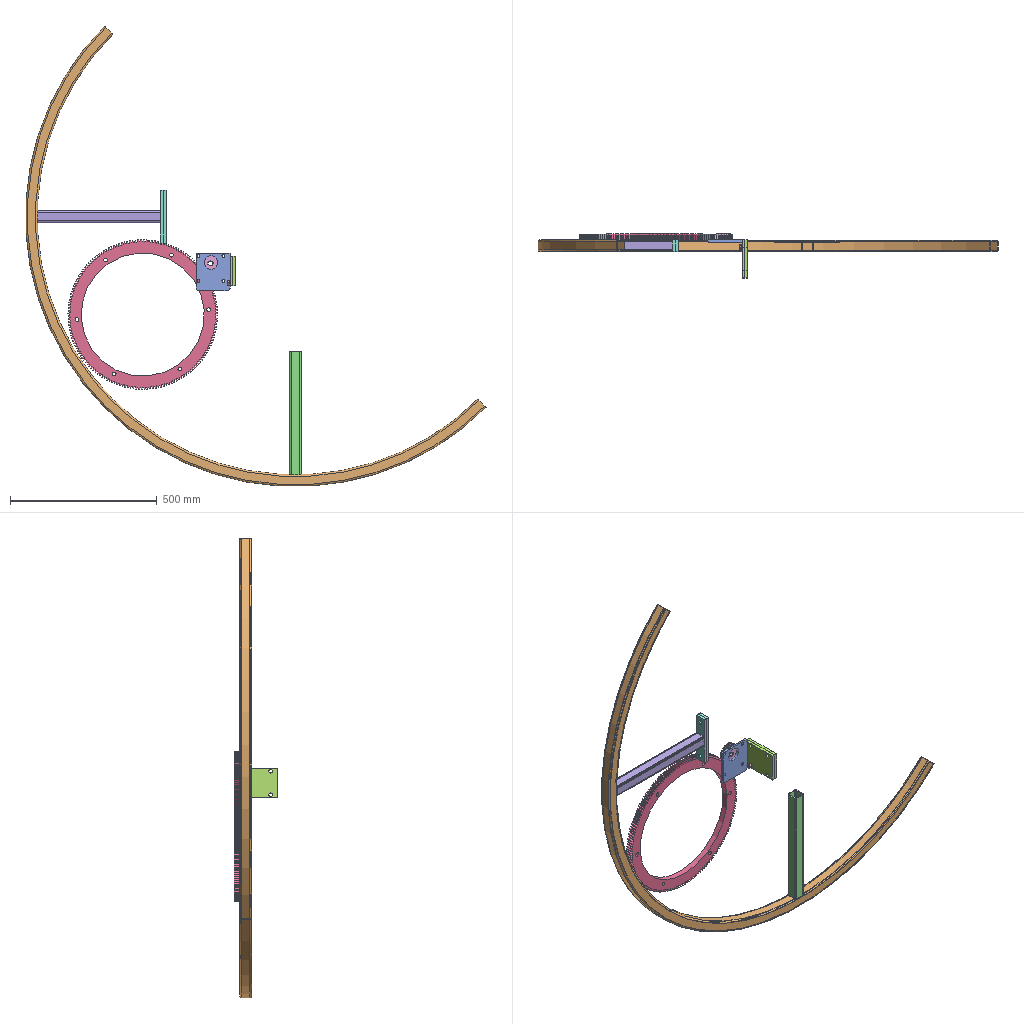Assembly | SolidWorks | 7 different items | 9 placed | box 1569 x 150 x 1569 mm
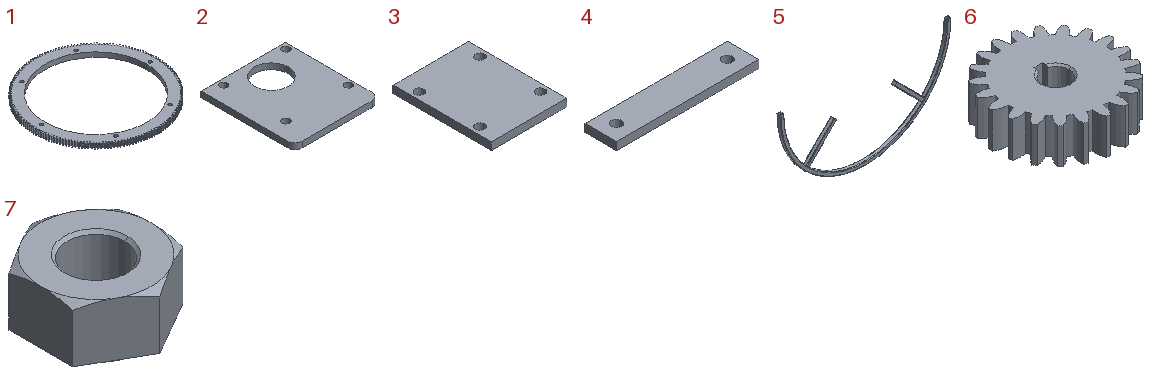Parts list (item | quantity | size | volume | features):
1 | x1 | 509.982 x 509.982 x 20 mm | 1197057 mm3 | features ICE 2, CirPattern 1, Extrusion 1, HoleWzd 1
2 | x1 | 115 x 128 x 8 mm | 101608 mm3 | features Chamfer 1, Extrusion 1, Fillet 1, HoleWzd 1, ICE 1
3 | x2 | 100 x 130 x 10 mm | 125476 mm3 | features Chamfer 1, Extrusion 1, HoleWzd 1
4 | x2 | 180 x 40 x 10 mm | 69345 mm3 | features HoleWzd 2, Extrusion 1
5 | x1 | 1840 x 40 x 920 mm | 1638745 mm3 | features WeldMemberFeat 1, WeldmentFeature 1
6 | x1 | 68.925 x 68.813 x 20 mm | 57301 mm3 | features ICE 2, Chamfer 1, CirPattern 1, Extrusion 1
7 | x1 | 16 x 18.475 x 8.4 mm | 1358 mm3 | features Cut 2, Chamfer 1, Extrusion 1
Mates (type | each side: item.copy, entity, surface, feature):
Symmetric | 5.1 face plane Gb/t 6728—2002 square hollow section 40×3.2(1) | 5.1 face plane Gb/t 6728—2002 square hollow section 40×3.2(1) | assembly plane | 2 times
Coincident | 5.1 face plane Gb/t 6728—2002 square hollow section 40×3.2(1) | 4.1 face plane Boss-Extrude1 | 2 times
DistanceDim | 4.1 face plane Boss-Extrude1 | 5.1 face plane Gb/t 6728—2002 square hollow section 40×3.2(1)
Coincident | 4.1 face plane Boss-Extrude1 | 4.2 face plane Boss-Extrude1 | 3 times
Concentric | 3.1 face cylinder Ø12 Hole1 | 7.1 face cylinder Extrude1
Coincident | 3.1 face plane Boss-Extrude1 | 7.1 face plane Extrude1
Coincident | 2.1 face plane Boss-Extrude1 | 3.1 face plane Boss-Extrude1 | 2 times
DistanceDim | 2.1 face plane Boss-Extrude1 | 3.1 face plane Boss-Extrude1
Coincident | 3.1 face plane Boss-Extrude1 | 3.2 face plane Boss-Extrude1 | 3 times
Coincident | 1.1 face plane Boss-Extrude1 | 6.1 face plane Boss-Extrude1
Coincident | 5.1 face plane Gb/t 6728—2002 square hollow section 40×3.2(1) | 1.1 face plane Boss-Extrude1
Coincident | 2.1 face plane Boss-Extrude1 | 6.1 face plane Boss-Extrude1